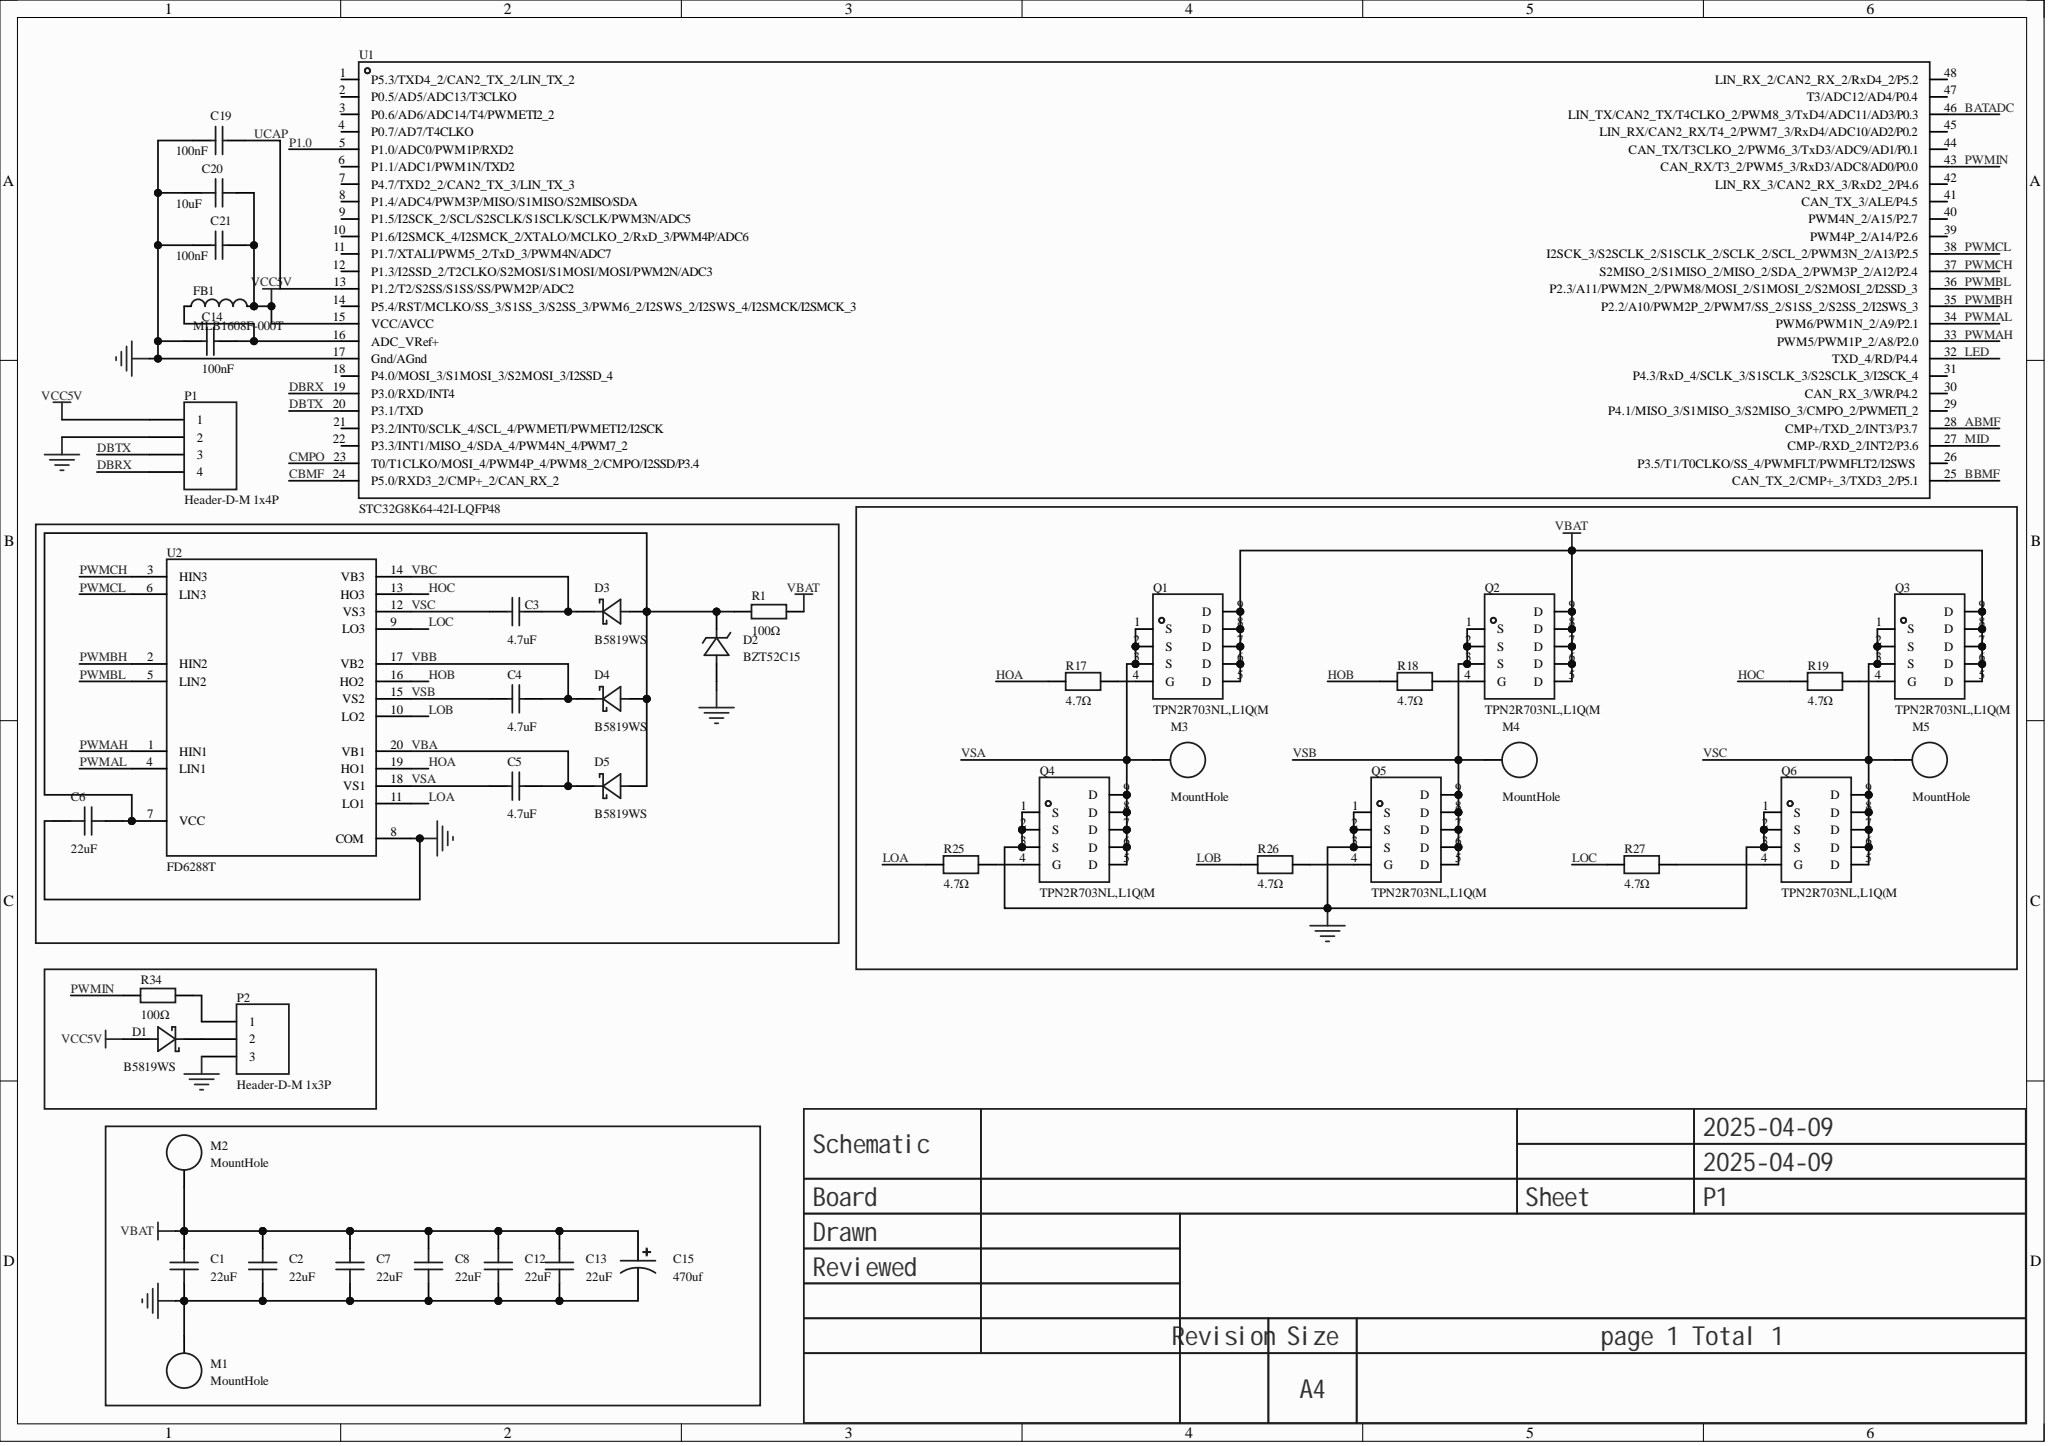Circuit board | Altium Designer | 66 parts | 43 nets
Bill of materials:
Comment,Description,Designator,Footprint,LibRef,Quantity
"22uF","Capacitance:22uF;Tolerance:±20%;Rated voltage:25V;Dielectric (temp. coefficient):X5R;","C1, C2, C6, C7, C8, C9, C12, C13","C0805","CL21A226MAQNNNE","8"
"4.7uF","Capacitance:4.7uF;Tolerance:±10%;Rated voltage:25V;Dielectric (temp. coefficient):X5R;","C3, C4, C5","C0805","CL21A475KAQNNNE","3"
"10uF","Capacitance:10uF;Tolerance:±10%;Rated voltage:10V;Temperature coefficient:X5R;","C10, C20","C0603","CGA0603X5R106K100JT","2"
"100nF","Capacitance:100nF;Tolerance:±10%;Rated voltage:16V;Dielectric (temp. coefficient):X7R;","C11, C14, C18, C19, C21","C0603","CL10B104KO8NNNC","5"
"470uf","","C15","焊盘","470uf","1"
"100nF","Capacitance:100nF;Tolerance:±10%;Rated voltage:16V;Dielectric (temp. coefficient):X7R;","C27, C28, C29","C0402","CL05B104KO5NNNC","3"
"B5819WS","Diode configuration:Single;Forward voltage(Vf):600mV@1.0A;DC reverse voltage(Vr):40V;Rectified current:1A;","D1, D3, D4, D5","SOD-323_L1.7-W1.3-LS2.5-FD","B5819WS_C7420331","4"
"BZT52C15","Diode configuration:Single;Zener voltage (nominal):15V;Zener voltage (range):14.25V~15.75V;Power dissipation(Pd):500mW;","D2","SOD-123_L2.7-W1.6-LS3.7-RD","BZT52C15_C19077412","1"
"DSK34","Diode configuration:Single;Forward voltage(Vf):550mV@3A;DC reverse voltage(Vr):40V;Rectified current:3A;","D6","SOD-123_L2.8-W1.8-LS3.7-RD","DSK34_C41029","1"
"MLB1608F-000T","Impedance@frequency:0Ω@100MHz;Tolerance:±25%;DC resistance(DCR):-;","FB1","L0603","MLB1608F-000T","1"
"MountHole","Mounting hole","M1, M2, M3, M4, M5","3*4焊盘","MountHole","5"
"Header-D-M 1x4P","1x4pin, through-hole, pin header","P1","调试端口2.54_1X4","Header-D-M 1x4P","1"
"Header-D-M 1x3P","1x3pin, through-hole, pin header","P2","3P","Header-D-M 1x3P","1"
"TPN2R703NL,L1Q(M","Type:1 N-channel;Drain-source voltage(Vdss):30V;Continuous drain current(Id):-;On-resistance(RDS(on)@Vgs,Id):3.3mΩ@4.5V,22.5A;Power:42W;Threshold voltage(Vgs(th)@Id):1.3V@0.3mA;","Q1, Q2, Q3, Q4, Q5, Q6","TSON-8_L3.1-W3.1-P0.65-LS3.3-BL-EP","TPN2R703NL,L1Q(M","6"
"100Ω","Resistor type:Thick film resistor;Resistance:100Ω;Tolerance:±1%;Power:100mW;Max working voltage:75V;Temperature coefficient:±200ppm/?;","R1, R34","R0603","0603WAF1000T5E","2"
"10kΩ","Resistor type:Thick film resistor;Resistance:10kΩ;Tolerance:±1%;Power:100mW;Max working voltage:75V;Temperature coefficient:±100ppm/?;","R2, R35","R0603","0603WAF1002T5E","2"
"4.7Ω","Resistor type:Thick film resistor;Resistance:4.7Ω;Tolerance:±5%;Power:100mW;Working voltage:75V;Temperature coefficient:±200ppm/?;","R17, R18, R19, R25, R26, R27","R0603","FRC0603J4R7 TS","6"
"47kΩ","Resistor type:Thick film resistor;Resistance:47kΩ;Tolerance:±1%;Power:100mW;Max working voltage:75V;Temperature coefficient:±100ppm/?;","R33","R0603","FRC0603F4702TS","1"
"5.1kΩ","Resistor type:Thick film resistor;Resistance:5.1kΩ;Tolerance:±1%;Power:100mW;Max working voltage:75V;Temperature coefficient:±100ppm/?;","R41, R43, R45","R0603","0603WAF5101T5E","3"
"1kΩ","Resistor type:Thick film resistor;Resistance:1kΩ;Tolerance:±1%;Power:100mW;Max working voltage:75V;Temperature coefficient:±100ppm/?;","R42, R44, R46, R51, R52, R53","R0603","0603WAF1001T5E","6"
"LTST-C191KSKT","","STA","LED0603-RD-YELLOW","LTST-C191KSKT","1"
"STC32G8K64-42I-LQFP48","","U1","LQFP-48_L7.0-W7.0-P0.50-LS9.0-BL","STC32G8K64-42I-LQFP48","1"
"FD6288T","Three independent half-bridge gate driver ICs","U2","TSSOP-20_L6.5-W4.4-P0.65-LS6.4-BL","FD6288T","1"
"SE8650KX-LF","","U3","SOT-89-3_L4.3-W2.3-P1.50-LS4.3-BR","SE8650KX-LF","1"
Netlist (Protel format):
[
C1
C0805
22uF



]
[
C2
C0805
22uF



]
[
C3
C0805
4.7uF



]
[
C4
C0805
4.7uF



]
[
C5
C0805
4.7uF



]
[
C6
C0805
22uF



]
[
C7
C0805
22uF



]
[
C8
C0805
22uF



]
[
C9
C0805
22uF



]
[
C10
C0603
10uF



]
[
C11
C0603
100nF



]
[
C12
C0805
22uF



]
[
C13
C0805
22uF



]
[
C14
C0603
100nF



]
[
C15
焊盘
470uf



]
[
C18
C0603
100nF



]
[
C19
C0603
100nF



]
[
C20
C0603
10uF



]
[
C21
C0603
100nF



]
[
C27
C0402
100nF



]
[
C28
C0402
100nF



]
[
C29
C0402
100nF



]
[
D1
SOD-323_L1.7-W1.3-LS2.5-FD
B5819WS



]
[
D2
SOD-123_L2.7-W1.6-LS3.7-RD
BZT52C15



]
[
D3
SOD-323_L1.7-W1.3-LS2.5-FD
B5819WS



]
[
D4
SOD-323_L1.7-W1.3-LS2.5-FD
B5819WS



]
[
D5
SOD-323_L1.7-W1.3-LS2.5-FD
B5819WS



]
[
D6
SOD-123_L2.8-W1.8-LS3.7-RD
DSK34



]
[
FB1
L0603
MLB1608F-000T



]
[
M1
3*4焊盘
MountHole



]
[
M2
3*4焊盘
MountHole



]
[
M3
3*4焊盘
MountHole



]
[
M4
3*4焊盘
MountHole



]
[
M5
3*4焊盘
MountHole



]
[
P1
调试端口2.54_1X4
Header-D-M 1x4P



]
[
P2
3P
Header-D-M 1x3P



]
[
Q1
TSON-8_L3.1-W3.1-P0.65-LS3.3-BL-EP
TPN2R703NL,L1Q(M



]
[
Q2
TSON-8_L3.1-W3.1-P0.65-LS3.3-BL-EP
TPN2R703NL,L1Q(M



]
[
Q3
TSON-8_L3.1-W3.1-P0.65-LS3.3-BL-EP
TPN2R703NL,L1Q(M



]
[
Q4
TSON-8_L3.1-W3.1-P0.65-LS3.3-BL-EP
TPN2R703NL,L1Q(M



]
[
Q5
TSON-8_L3.1-W3.1-P0.65-LS3.3-BL-EP
TPN2R703NL,L1Q(M



]
[
Q6
TSON-8_L3.1-W3.1-P0.65-LS3.3-BL-EP
TPN2R703NL,L1Q(M



]
[
R1
R0603
100Ω



]
[
R2
R0603
10kΩ



]
[
R17
R0603
4.7Ω



]
[
R18
R0603
4.7Ω



]
[
R19
R0603
4.7Ω



]
[
R25
R0603
4.7Ω



]
[
R26
R0603
4.7Ω



]
[
R27
R0603
4.7Ω



]
[
R33
R0603
47kΩ



]
[
R34
R0603
100Ω



]
[
R35
R0603
10kΩ



]
[
R41
R0603
5.1kΩ



]
[
R42
R0603
1kΩ



]
[
R43
R0603
5.1kΩ



]
[
R44
R0603
1kΩ



]
[
R45
R0603
5.1kΩ



]
[
R46
R0603
1kΩ



]
[
R51
R0603
1kΩ



]
[
R52
R0603
1kΩ



]
[
R53
R0603
1kΩ



]
[
STA
LED0603-RD-YELLOW
LTST-C191KSKT



]
[
U1
LQFP-48_L7.0-W7.0-P0.50-LS9.0-BL
STC32G8K64-42I-LQFP48



]
[
U2
TSSOP-20_L6.5-W4.4-P0.65-LS6.4-BL
FD6288T



]
[
U3
SOT-89-3_L4.3-W2.3-P1.50-LS4.3-BR
SE8650KX-LF



]
(
VSC
C3-1
M5-1
Q3-1
Q3-2
Q3-3
Q6-5
Q6-6
Q6-7
Q6-8
Q6-9
R45-2
U2-12
)
(
VSB
C4-1
M4-1
Q2-1
Q2-2
Q2-3
Q5-5
Q5-6
Q5-7
Q5-8
Q5-9
R43-2
U2-15
)
(
VSA
C5-1
M3-1
Q1-1
Q1-2
Q1-3
Q4-5
Q4-6
Q4-7
Q4-8
Q4-9
R41-2
U2-18
)
(
VCC5V
C10-2
C11-2
C20-2
C21-2
D1-1
FB1-2
P1-1
STA-2
U1-15
U3-3
)
(
VBC
C3-2
D3-2
U2-14
)
(
VBB
C4-2
D4-2
U2-17
)
(
VBAT
C1-2
C2-2
C7-2
C8-2
C12-2
C13-2
C15-1
D6-2
M2-1
Q1-5
Q1-6
Q1-7
Q1-8
Q1-9
Q2-5
Q2-6
Q2-7
Q2-8
Q2-9
Q3-5
Q3-6
Q3-7
Q3-8
Q3-9
R1-2
R33-2
)
(
VBA
C5-2
D5-2
U2-20
)
(
UCAP
C19-2
U1-13
)
(
PWMIN
R34-1
U1-43
)
(
PWMCL
U1-38
U2-6
)
(
PWMCH
U1-37
U2-3
)
(
PWMBL
U1-36
U2-5
)
(
PWMBH
U1-35
U2-2
)
(
PWMAL
U1-34
U2-4
)
(
PWMAH
U1-33
U2-1
)
(
NetR2_2
R2-2
STA-1
)
(
NetQ6_4
Q6-4
R27-2
)
(
NetQ5_4
Q5-4
R26-2
)
(
NetQ4_4
Q4-4
R25-2
)
(
NetQ3_4
Q3-4
R19-2
)
(
NetQ2_4
Q2-4
R18-2
)
(
NetQ1_4
Q1-4
R17-2
)
(
NetP2_1
P2-1
R34-2
)
(
NetD1_2
D1-2
P2-2
)
(
NetC14_2
C14-2
FB1-1
U1-16
)
(
NetC9_2
C9-2
D6-1
U3-2
)
(
NetC6_2
C6-2
D2-1
D3-1
D4-1
D5-1
R1-1
U2-7
)
(
MID
R42-2
R44-2
R46-2
U1-27
)
(
LOC
R27-1
U2-9
)
(
LOB
R26-1
U2-10
)
(
LOA
R25-1
U2-11
)
(
LED
R2-1
U1-32
)
(
HOC
R19-1
U2-13
)
(
HOB
R18-1
U2-16
)
(
HOA
R17-1
U2-19
)
(
GND
C1-1
C2-1
C6-1
C7-1
C8-1
C9-1
C10-1
C11-1
C12-1
C13-1
C14-1
C15-2
C18-1
C19-1
C20-1
C21-1
C27-1
C28-1
C29-1
D2-2
M1-1
P1-2
P2-3
Q4-1
Q4-2
Q4-3
Q5-1
Q5-2
Q5-3
Q6-1
Q6-2
Q6-3
R35-1
R51-1
R52-1
R53-1
U1-17
U2-8
U3-1
)
(
DBTX
P1-3
U1-20
)
(
DBRX
P1-4
U1-19
)
(
CBMF
C29-2
R45-1
R46-1
R53-2
U1-24
)
(
BBMF
C28-2
R43-1
R44-1
R52-2
U1-25
)
(
BATADC
C18-2
R33-1
R35-2
U1-46
)
(
ABMF
C27-2
R41-1
R42-1
R51-2
U1-28
)